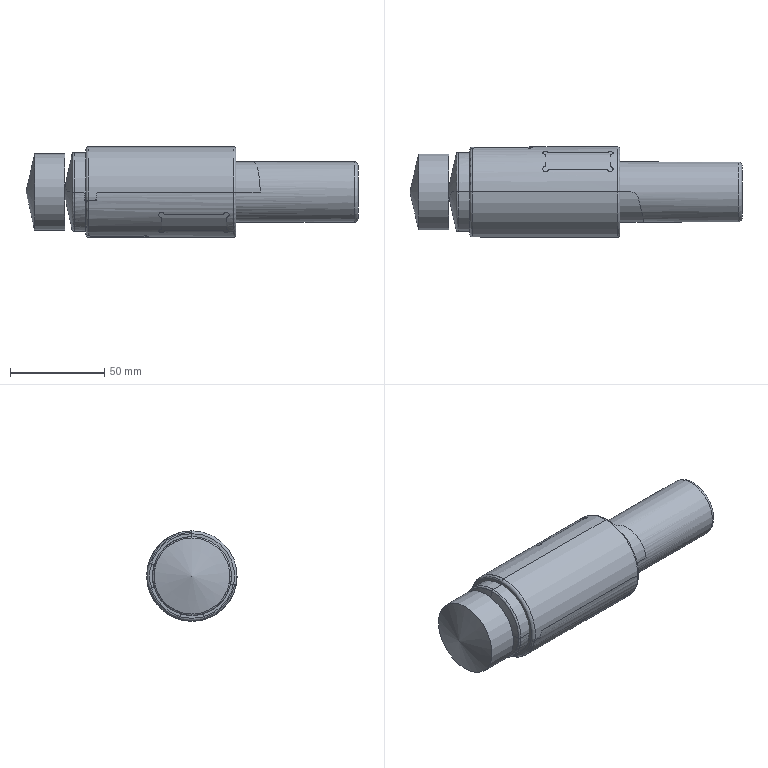NC program | NX | posted with a generic post | part box 176.413 x 48 x 48 mm
Whole program:
N10 G17 G21 G94 G90
(ZLEVEL_PROFILE_1 , TOOL : D6JING)
N12 T08 M6
N14 G54
N16 G17 G0 G90 X-57.935 Y-8.811 S5000 M3
N18 G43 Z33.873 H8
N20 Z19.5
N22 G94 G1 Z18. F1000.
N24 X-57.274 Y-8.184
N26 G3 X-57.104 Y-7.608 R0.6
N28 G1 X-58.032 Y-3.753
N30 G3 X-58.931 Y-3.002 R0.999
N32 G1 X-58.993 Y-3.
N34 X-153.33
N36 X-155.89 Y-2.996
N38 G3 X-156.41 Y-3.295 R0.6
N40 G1 X-156.848 Y-4.051
N42 Z19.5
N44 G0 Z34.765
N46 X-145.635 Y-5.559 Z34.556
N48 X-134.423 Y-7.058 Z34.281
N50 X-123.21 Y-8.542 Z33.942
N52 X-111.998 Y-10.011 Z33.538
N54 X-100.786 Y-11.461 Z33.07
N56 X-89.573 Y-12.889 Z32.54
N58 X-78.361 Y-14.292 Z31.949
N60 X-67.148 Y-15.669 Z31.297
N62 X-55.936 Y-17.016 Z30.585
N64 Z13.5
N66 G1 Z12.
N68 X-55.293 Y-16.399
N70 G3 X-55.126 Y-15.823 R0.6
N72 G1 X-55.23 Y-15.401
N74 X-58.036 Y-3.734
N76 G3 X-59. Y-3. R1.
N78 G1 X-153.341
N80 X-157.232 Y-2.996
N82 G3 X-157.752 Y-3.296 R0.6
N84 G1 X-158.19 Y-4.054
N86 Z13.5
N88 G0 Z34.764
N90 M5
N92 M2